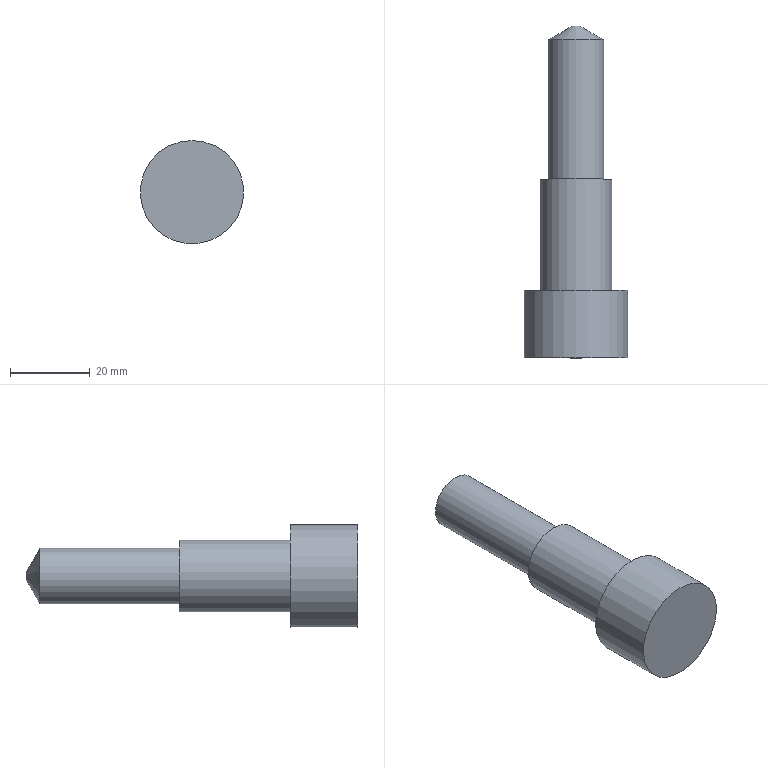Part | STEP file | solid 168 | 1 solid | 8 faces | box 26 x 83.5 x 26 mm | volume 21746 mm3 | plane 4 | cylinder 3 | cone 1 | commonest cylinder face diameters 14 x1 18 x1 26 x1